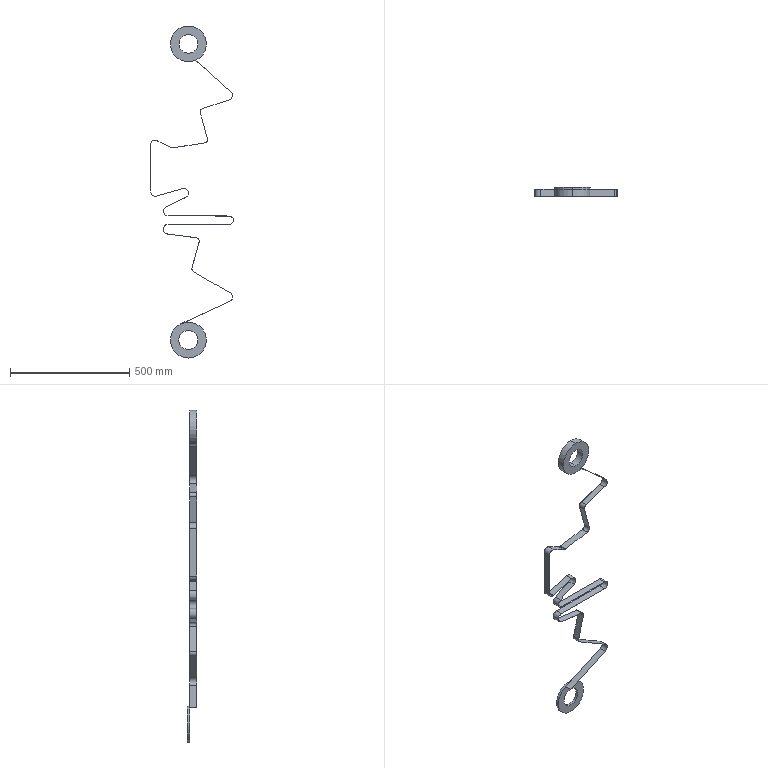Part | STEP file | Pay-off roll | 3 solids | 78 faces | box 345.65 x 40 x 1390 mm | volume 521219 mm3 | cylinder 40 | plane 38 | commonest cylinder face diameters 40 x7 39.8 x5 30 x4 35 x4 150 x4 35.2 x3